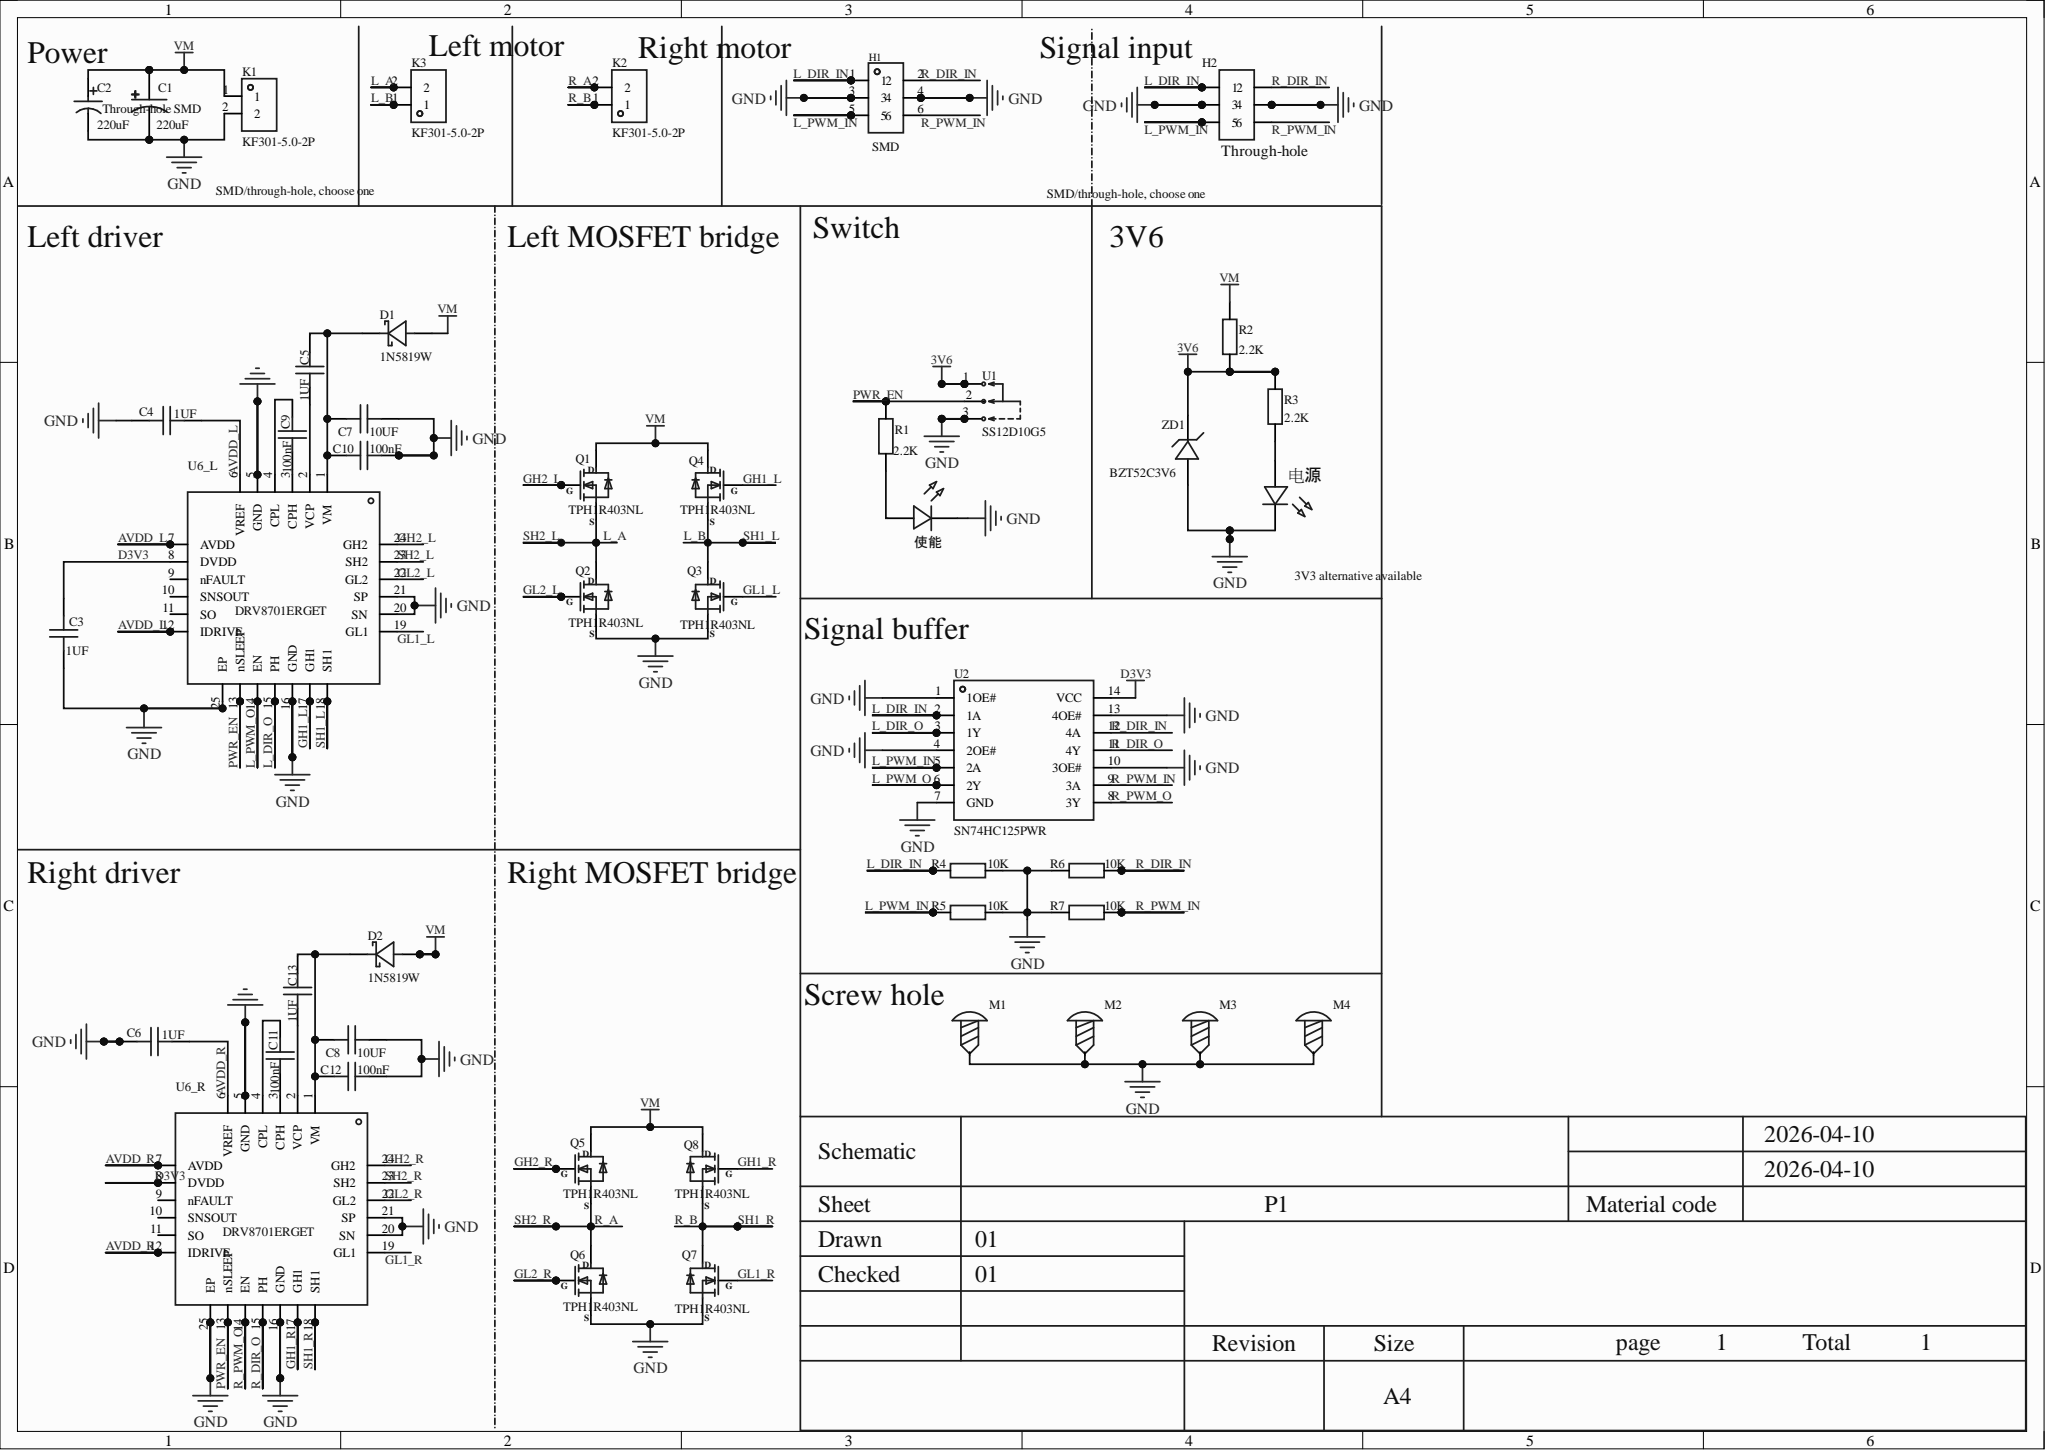Circuit board | Altium Designer | 46 parts | 37 nets
Bill of materials:
Comment,Description,Designator,Footprint,LibRef,Quantity
"220uF","Capacitance:220uF;Tolerance:±20%;Rated voltage:50V;Ripple current:670mA@100kHz;ESR:180mO@100kHz;","C1","CAP-SMD_BD8.0-L8.3-W8.3-FD","EEEFT1H221GP","1"
"220uF","Capacitance:220uF;Tolerance:±20%;Rated voltage:35V;","C2","CAP-TH_BD8.0-P3.50-D0.6-FD","ERS1VM221F12OT","1"
"1UF","","C3, C4, C5, C6, C13","C0603","CAP_0603","5"
"10UF","","C7, C8","C0603","CAP_0603","2"
"100nF","","C9, C10, C11, C12","C0603","CAP_0603","4"
"1N5819W","Diode configuration:-;Forward voltage (Vf):900mV@3A;DC reverse voltage (Vr):40V;Average rectified current (Io):1A;","D1, D2","SOD-123_L2.7-W1.6-LS3.7-RD-1","1N5819W","2"
"SMD","Pin structure:-;Pitch:2.54mm;Row spacing:-;Round/square pin:-;Mounting type:-;Rows:double row;Total pins:6P;Rated current:-;Rated voltage:-;Mating pin length:-;Plastic height:-;Contact material:-;Contact plating:-;Color:black;","H1","HDR-SMD_6P-P2.54-V-M-R2-C5-S7.4","2.54-2*3P立贴针","1"
"","","H2","HDR-TH_6P-P2.54-V-R2-C3-S2.54_A2541WV-2X3P","HDR-M_2.54_2x3","1"
"KF301-5.0-2P","Structure:1x2P;Pitch:5mm;Color:blue;Mounting:through-hole;Rated current:17A;Rated voltage:250V;Rows:1;Wire gauge - AWG:14~22;Wire gauge - mm2:1.5;Pins per row:2;Operating temperature:-30℃~+120℃;","K1, K2, K3","CONN-TH_P5.00_KF301-5.0-2P","KF301-5.0-2P","3"
"","","M1, M2, M3, M4","M4螺丝","M4螺丝","4"
"TPH1R403NL","","Q1, Q2, Q3, Q4, Q5, Q6, Q7, Q8","DFN5x6","TPH1R403NL","8"
"2.2K","","R1, R2, R3","R0603","Res_0603","3"
"10K","","R4, R5, R6, R7","R0603","Res_0603","4"
"SS12D10G5","电路结构:单刀双掷;安装方式:直插;额定电流(DC):2A;额定电压(DC):125V;机械寿命:3千次;","U1","SW-TH_SHOU-HAN_SS12D10G4","SS12D10G5","1"
"SN74HC125PWR","Input type:-;Supply voltage:2V~6V;Number of elements:4;Bits per element:1;Sink current (IOL):7.8mA;Source current (IOH):7.8mA;","U2","TSSOP-14_L5.0-W4.4-P0.65-LS6.5-BL","SN74HC125PWR","1"
"DRV8701ERGET","DRV8701 47V H-bridge smart gate driver","U6_L, U6_R","VQFN-24_L4.0-W4.0-P0.50-BL-EP2.5","DRV8701ERGET","2"
"BZT52C3V6","Diode configuration:single;Zener voltage (nominal):3.6V;Zener voltage (range):3.4V~3.8V;Power:350mW;Tolerance:-;","ZD1","SOD-123_L2.8-W1.8-LS3.7-RD","BZT52C3V6_C2113","1"
"","","使能, 电源","LED_0603","LED_0603-G, LED_0603-R","2"
Netlist (Protel format):
[
C1
CAP-SMD_BD8.0-L8.3-W8.3-FD
220uF



]
[
C2
CAP-TH_BD8.0-P3.50-D0.6-FD
220uF



]
[
C3
C0603
1UF



]
[
C4
C0603
1UF



]
[
C5
C0603
1UF



]
[
C6
C0603
1UF



]
[
C7
C0603
10UF



]
[
C8
C0603
10UF



]
[
C9
C0603
100nF



]
[
C10
C0603
100nF



]
[
C11
C0603
100nF



]
[
C12
C0603
100nF



]
[
C13
C0603
1UF



]
[
D1
SOD-123_L2.7-W1.6-LS3.7-RD-1
1N5819W



]
[
D2
SOD-123_L2.7-W1.6-LS3.7-RD-1
1N5819W



]
[
H1
HDR-SMD_6P-P2.54-V-M-R2-C5-S7.4
SMD



]
[
H2
HDR-TH_6P-P2.54-V-R2-C3-S2.54_A2541WV-2X3P




]
[
K1
CONN-TH_P5.00_KF301-5.0-2P
KF301-5.0-2P



]
[
K2
CONN-TH_P5.00_KF301-5.0-2P
KF301-5.0-2P



]
[
K3
CONN-TH_P5.00_KF301-5.0-2P
KF301-5.0-2P



]
[
M1
M4螺丝




]
[
M2
M4螺丝




]
[
M3
M4螺丝




]
[
M4
M4螺丝




]
[
Q1
DFN5x6
TPH1R403NL



]
[
Q2
DFN5x6
TPH1R403NL



]
[
Q3
DFN5x6
TPH1R403NL



]
[
Q4
DFN5x6
TPH1R403NL



]
[
Q5
DFN5x6
TPH1R403NL



]
[
Q6
DFN5x6
TPH1R403NL



]
[
Q7
DFN5x6
TPH1R403NL



]
[
Q8
DFN5x6
TPH1R403NL



]
[
R1
R0603
2.2K



]
[
R2
R0603
2.2K



]
[
R3
R0603
2.2K



]
[
R4
R0603
10K



]
[
R5
R0603
10K



]
[
R6
R0603
10K



]
[
R7
R0603
10K



]
[
U1
SW-TH_SHOU-HAN_SS12D10G4
SS12D10G5



]
[
U2
TSSOP-14_L5.0-W4.4-P0.65-LS6.5-BL
SN74HC125PWR



]
[
U6_L
VQFN-24_L4.0-W4.0-P0.50-BL-EP2.5
DRV8701ERGET



]
[
U6_R
VQFN-24_L4.0-W4.0-P0.50-BL-EP2.5
DRV8701ERGET



]
[
ZD1
SOD-123_L2.8-W1.8-LS3.7-RD
BZT52C3V6



]
[
使能
LED_0603




]
[
电源
LED_0603




]
(
VM
C1-1
C2-1
D1-2
D2-2
K1-1
Q1-1
Q4-1
Q5-1
Q8-1
R2-2
)
(
R_PWM_O
U2-8
U6_R-14
)
(
R_PWM_IN
H1-6
H2-6
R7-2
U2-9
)
(
R_DIR_O
U2-11
U6_R-15
)
(
R_DIR_IN
H1-2
H2-2
R6-2
U2-12
)
(
R_B
K2-1
Q7-1
Q8-3
U6_R-18
)
(
R_A
K2-2
Q5-3
Q6-1
U6_R-23
)
(
PWR_EN
R1-2
U1-2
U6_L-13
U6_R-13
)
(
NetR3_1
R3-1
电源-2
)
(
NetR1_1
R1-1
使能-2
)
(
NetC13_2
C13-2
U6_R-2
)
(
NetC11_2
C11-2
U6_R-4
)
(
NetC11_1
C11-1
U6_R-3
)
(
NetC9_2
C9-2
U6_L-4
)
(
NetC9_1
C9-1
U6_L-3
)
(
NetC8_1
C8-1
C12-1
C13-1
D2-1
U6_R-1
)
(
NetC5_2
C5-2
U6_L-2
)
(
NetC5_1
C5-1
C7-1
C10-1
D1-1
U6_L-1
)
(
L_PWM_O
U2-6
U6_L-14
)
(
L_PWM_IN
H1-5
H2-5
R5-1
U2-5
)
(
L_DIR_O
U2-3
U6_L-15
)
(
L_DIR_IN
H1-1
H2-1
R4-1
U2-2
)
(
L_B
K3-1
Q3-1
Q4-3
U6_L-18
)
(
L_A
K3-2
Q1-3
Q2-1
U6_L-23
)
(
GND
C1-2
C2-2
C3-1
C4-2
C6-2
C7-2
C8-2
C10-2
C12-2
H1-3
H1-4
H2-3
H2-4
K1-2
M1-1
M2-1
M3-1
M4-1
Q2-3
Q3-3
Q6-3
Q7-3
R4-2
R5-2
R6-1
R7-1
U1-3
U2-1
U2-4
U2-7
U2-10
U2-13
U6_L-5
U6_L-16
U6_L-20
U6_L-21
U6_L-25
U6_R-5
U6_R-16
U6_R-20
U6_R-21
U6_R-25
ZD1-2
使能-1
电源-1
)
(
GL2_R
Q6-2
U6_R-22
)
(
GL2_L
Q2-2
U6_L-22
)
(
GL1_R
Q7-2
U6_R-19
)
(
GL1_L
Q3-2
U6_L-19
)
(
GH2_R
Q5-2
U6_R-24
)
(
GH2_L
Q1-2
U6_L-24
)
(
GH1_R
Q8-2
U6_R-17
)
(
GH1_L
Q4-2
U6_L-17
)
(
D3V3
C3-2
U2-14
U6_L-8
U6_R-8
)
(
AVDD_R
C6-1
U6_R-6
U6_R-7
U6_R-12
)
(
AVDD_L
C4-1
U6_L-6
U6_L-7
U6_L-12
)
(
3V6
R2-1
R3-2
U1-1
ZD1-1
)